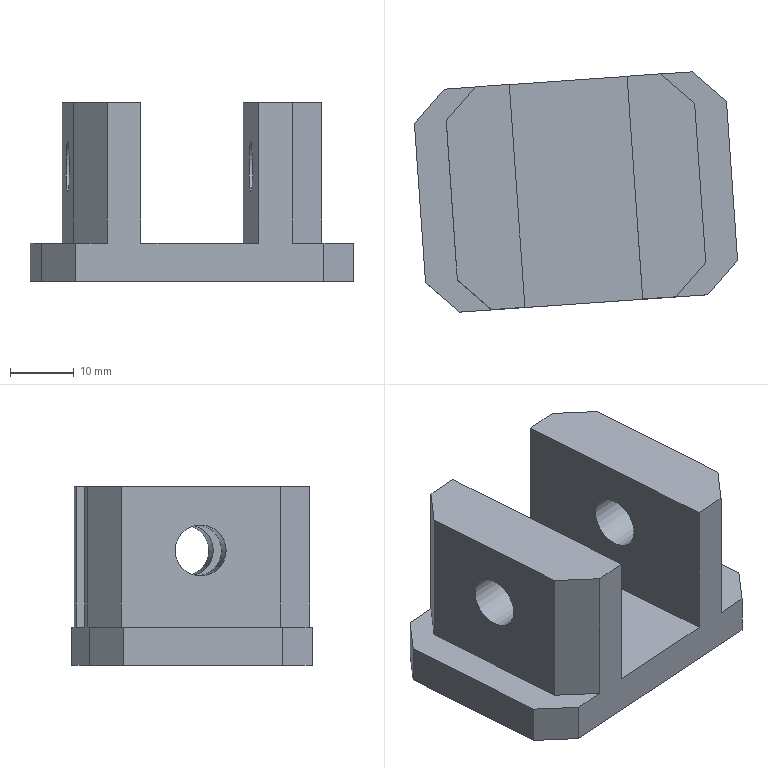Part | STEP file | 车灯-后视镜_id362_x_t | 1 solid | 24 faces | box 50.625 x 37.635 x 28 mm | volume 23645 mm3 | plane 22 | cylinder 2 | commonest cylinder face diameters 8 x2
STEP:
#1=CARTESIAN_POINT('',(14.203,-0.1524,-249.5));
#2=VERTEX_POINT('',#1);
#3=CARTESIAN_POINT('',(-4.252,-1.443,-249.5));
#4=VERTEX_POINT('',#3);
#5=CARTESIAN_POINT('',(22.932,0.458,-249.5));
#6=DIRECTION('',(-0.9976,-0.06976,0.));
#7=VECTOR('',#6,1.);
#8=LINE('',#5,#7);
#9=EDGE_CURVE('',#2,#4,#8,.T.);
#10=ORIENTED_EDGE('',*,*,#9,.T.);
#11=CARTESIAN_POINT('',(-1.81,-36.358,-249.5));
#12=VERTEX_POINT('',#11);
#13=CARTESIAN_POINT('',(-3.417,-13.382,-249.5));
#14=DIRECTION('',(-0.06976,0.9976,0.));
#15=VECTOR('',#14,1.);
#16=LINE('',#13,#15);
#17=EDGE_CURVE('',#12,#4,#16,.T.);
#18=ORIENTED_EDGE('',*,*,#17,.F.);
#19=CARTESIAN_POINT('',(16.645,-35.067,-249.5));
#20=VERTEX_POINT('',#19);
#21=CARTESIAN_POINT('',(25.373,-34.457,-249.5));
#22=DIRECTION('',(0.9976,0.06976,0.));
#23=VECTOR('',#22,1.);
#24=LINE('',#21,#23);
#25=EDGE_CURVE('',#12,#20,#24,.T.);
#26=ORIENTED_EDGE('',*,*,#25,.T.);
#27=CARTESIAN_POINT('',(15.038,-12.092,-249.5));
#28=DIRECTION('',(0.06976,-0.9976,0.));
#29=VECTOR('',#28,1.);
#30=LINE('',#27,#29);
#31=EDGE_CURVE('',#2,#20,#30,.T.);
#32=ORIENTED_EDGE('',*,*,#31,.F.);
#33=EDGE_LOOP('',(#10,#18,#26,#32));
#34=FACE_OUTER_BOUND('',#33,.T.);
#35=CARTESIAN_POINT('',(23.294,-4.723,-249.5));
#36=DIRECTION('',(0.,0.,1.));
#37=DIRECTION('',(0.06976,-0.9976,0.));
#38=AXIS2_PLACEMENT_3D('',#35,#36,#37);
#39=PLANE('',#38);
#40=ADVANCED_FACE('',(#34),#39,.T.);
#41=CARTESIAN_POINT('',(24.428,0.5626,-249.5));
#42=VERTEX_POINT('',#41);
#43=CARTESIAN_POINT('',(19.44,0.2139,-249.5));
#44=VERTEX_POINT('',#43);
#45=CARTESIAN_POINT('',(11.959,-0.3093,-249.5));
#46=DIRECTION('',(-0.9976,-0.06976,0.));
#47=VECTOR('',#46,1.);
#48=LINE('',#45,#47);
#49=EDGE_CURVE('',#42,#44,#48,.T.);
#50=ORIENTED_EDGE('',*,*,#49,.T.);
#51=CARTESIAN_POINT('',(24.777,-4.425,-249.5));
#52=VERTEX_POINT('',#51);
#53=CARTESIAN_POINT('',(19.44,0.2139,-249.5));
#54=DIRECTION('',(-0.7547,0.6561,0.));
#55=VECTOR('',#54,1.);
#56=LINE('',#53,#55);
#57=EDGE_CURVE('',#52,#44,#56,.T.);
#58=ORIENTED_EDGE('',*,*,#57,.F.);
#59=CARTESIAN_POINT('',(26.521,-29.364,-249.5));
#60=VERTEX_POINT('',#59);
#61=CARTESIAN_POINT('',(25.589,-16.037,-249.5));
#62=DIRECTION('',(-0.06976,0.9976,0.));
#63=VECTOR('',#62,1.);
#64=LINE('',#61,#63);
#65=EDGE_CURVE('',#60,#52,#64,.T.);
#66=ORIENTED_EDGE('',*,*,#65,.F.);
#67=CARTESIAN_POINT('',(21.882,-34.701,-249.5));
#68=VERTEX_POINT('',#67);
#69=CARTESIAN_POINT('',(26.521,-29.364,-249.5));
#70=DIRECTION('',(0.6561,0.7547,0.));
#71=VECTOR('',#70,1.);
#72=LINE('',#69,#71);
#73=EDGE_CURVE('',#68,#60,#72,.T.);
#74=ORIENTED_EDGE('',*,*,#73,.F.);
#75=CARTESIAN_POINT('',(26.87,-34.352,-249.5));
#76=VERTEX_POINT('',#75);
#77=CARTESIAN_POINT('',(14.4,-35.224,-249.5));
#78=DIRECTION('',(0.9976,0.06976,0.));
#79=VECTOR('',#78,1.);
#80=LINE('',#77,#79);
#81=EDGE_CURVE('',#68,#76,#80,.T.);
#82=ORIENTED_EDGE('',*,*,#81,.T.);
#83=CARTESIAN_POINT('',(31.509,-29.015,-249.5));
#84=VERTEX_POINT('',#83);
#85=CARTESIAN_POINT('',(31.509,-29.015,-249.5));
#86=DIRECTION('',(-0.6561,-0.7547,0.));
#87=VECTOR('',#86,1.);
#88=LINE('',#85,#87);
#89=EDGE_CURVE('',#84,#76,#88,.T.);
#90=ORIENTED_EDGE('',*,*,#89,.F.);
#91=CARTESIAN_POINT('',(29.765,-4.076,-249.5));
#92=VERTEX_POINT('',#91);
#93=CARTESIAN_POINT('',(29.778,-4.269,-249.5));
#94=DIRECTION('',(-0.06976,0.9976,0.));
#95=VECTOR('',#94,1.);
#96=LINE('',#93,#95);
#97=EDGE_CURVE('',#84,#92,#96,.T.);
#98=ORIENTED_EDGE('',*,*,#97,.T.);
#99=CARTESIAN_POINT('',(24.428,0.5626,-249.5));
#100=DIRECTION('',(0.7547,-0.6561,0.));
#101=VECTOR('',#100,1.);
#102=LINE('',#99,#101);
#103=EDGE_CURVE('',#42,#92,#102,.T.);
#104=ORIENTED_EDGE('',*,*,#103,.F.);
#105=EDGE_LOOP('',(#50,#58,#66,#74,#82,#90,#98,#104));
#106=FACE_OUTER_BOUND('',#105,.T.);
#107=CARTESIAN_POINT('',(12.321,-5.49,-249.5));
#108=DIRECTION('',(0.,0.,1.));
#109=DIRECTION('',(0.06976,-0.9976,0.));
#110=AXIS2_PLACEMENT_3D('',#107,#108,#109);
#111=PLANE('',#110);
#112=ADVANCED_FACE('',(#106),#111,.T.);
#113=CARTESIAN_POINT('',(-19.116,-7.494,-249.5));
#114=VERTEX_POINT('',#113);
#115=CARTESIAN_POINT('',(-17.372,-32.434,-249.5));
#116=VERTEX_POINT('',#115);
#117=CARTESIAN_POINT('',(-19.102,-7.687,-249.5));
#118=DIRECTION('',(0.06976,-0.9976,0.));
#119=VECTOR('',#118,1.);
#120=LINE('',#117,#119);
#121=EDGE_CURVE('',#114,#116,#120,.T.);
#122=ORIENTED_EDGE('',*,*,#121,.T.);
#123=CARTESIAN_POINT('',(-12.035,-37.073,-249.5));
#124=VERTEX_POINT('',#123);
#125=CARTESIAN_POINT('',(-12.035,-37.073,-249.5));
#126=DIRECTION('',(-0.7547,0.6561,0.));
#127=VECTOR('',#126,1.);
#128=LINE('',#125,#127);
#129=EDGE_CURVE('',#124,#116,#128,.T.);
#130=ORIENTED_EDGE('',*,*,#129,.F.);
#131=CARTESIAN_POINT('',(-7.048,-36.724,-249.5));
#132=VERTEX_POINT('',#131);
#133=CARTESIAN_POINT('',(35.349,-33.759,-249.5));
#134=DIRECTION('',(0.9976,0.06976,0.));
#135=VECTOR('',#134,1.);
#136=LINE('',#133,#135);
#137=EDGE_CURVE('',#124,#132,#136,.T.);
#138=ORIENTED_EDGE('',*,*,#137,.T.);
#139=CARTESIAN_POINT('',(-12.384,-32.085,-249.5));
#140=VERTEX_POINT('',#139);
#141=CARTESIAN_POINT('',(-7.048,-36.724,-249.5));
#142=DIRECTION('',(0.7547,-0.6561,0.));
#143=VECTOR('',#142,1.);
#144=LINE('',#141,#143);
#145=EDGE_CURVE('',#140,#132,#144,.T.);
#146=ORIENTED_EDGE('',*,*,#145,.F.);
#147=CARTESIAN_POINT('',(-14.128,-7.146,-249.5));
#148=VERTEX_POINT('',#147);
#149=CARTESIAN_POINT('',(-13.316,-18.757,-249.5));
#150=DIRECTION('',(0.06976,-0.9976,0.));
#151=VECTOR('',#150,1.);
#152=LINE('',#149,#151);
#153=EDGE_CURVE('',#148,#140,#152,.T.);
#154=ORIENTED_EDGE('',*,*,#153,.F.);
#155=CARTESIAN_POINT('',(-9.489,-1.809,-249.5));
#156=VERTEX_POINT('',#155);
#157=CARTESIAN_POINT('',(-14.128,-7.146,-249.5));
#158=DIRECTION('',(-0.6561,-0.7547,0.));
#159=VECTOR('',#158,1.);
#160=LINE('',#157,#159);
#161=EDGE_CURVE('',#156,#148,#160,.T.);
#162=ORIENTED_EDGE('',*,*,#161,.F.);
#163=CARTESIAN_POINT('',(-14.477,-2.158,-249.5));
#164=VERTEX_POINT('',#163);
#165=CARTESIAN_POINT('',(32.907,1.156,-249.5));
#166=DIRECTION('',(-0.9976,-0.06976,0.));
#167=VECTOR('',#166,1.);
#168=LINE('',#165,#167);
#169=EDGE_CURVE('',#156,#164,#168,.T.);
#170=ORIENTED_EDGE('',*,*,#169,.T.);
#171=CARTESIAN_POINT('',(-19.116,-7.494,-249.5));
#172=DIRECTION('',(0.6561,0.7547,0.));
#173=VECTOR('',#172,1.);
#174=LINE('',#171,#173);
#175=EDGE_CURVE('',#114,#164,#174,.T.);
#176=ORIENTED_EDGE('',*,*,#175,.F.);
#177=EDGE_LOOP('',(#122,#130,#138,#146,#154,#162,#170,#176));
#178=FACE_OUTER_BOUND('',#177,.T.);
#179=CARTESIAN_POINT('',(33.27,-4.025,-249.5));
#180=DIRECTION('',(0.,0.,1.));
#181=DIRECTION('',(0.06976,-0.9976,0.));
#182=AXIS2_PLACEMENT_3D('',#179,#180,#181);
#183=PLANE('',#182);
#184=ADVANCED_FACE('',(#178),#183,.T.);
#185=ORIENTED_EDGE('',*,*,#97,.F.);
#186=CARTESIAN_POINT('',(31.509,-29.015,-255.5));
#187=VERTEX_POINT('',#186);
#188=CARTESIAN_POINT('',(31.509,-29.015,-255.5));
#189=DIRECTION('',(0.,0.,1.));
#190=VECTOR('',#189,1.);
#191=LINE('',#188,#190);
#192=EDGE_CURVE('',#187,#84,#191,.T.);
#193=ORIENTED_EDGE('',*,*,#192,.F.);
#194=CARTESIAN_POINT('',(29.765,-4.076,-255.5));
#195=VERTEX_POINT('',#194);
#196=CARTESIAN_POINT('',(30.577,-15.688,-255.5));
#197=DIRECTION('',(0.06976,-0.9976,0.));
#198=VECTOR('',#197,1.);
#199=LINE('',#196,#198);
#200=EDGE_CURVE('',#195,#187,#199,.T.);
#201=ORIENTED_EDGE('',*,*,#200,.F.);
#202=CARTESIAN_POINT('',(29.765,-4.076,-255.5));
#203=DIRECTION('',(0.,0.,-1.));
#204=VECTOR('',#203,1.);
#205=LINE('',#202,#204);
#206=EDGE_CURVE('',#92,#195,#205,.T.);
#207=ORIENTED_EDGE('',*,*,#206,.F.);
#208=EDGE_LOOP('',(#185,#193,#201,#207));
#209=FACE_OUTER_BOUND('',#208,.T.);
#210=CARTESIAN_POINT('',(30.577,-15.688,-255.5));
#211=DIRECTION('',(0.9976,0.06976,0.));
#212=DIRECTION('',(0.,0.,-1.));
#213=AXIS2_PLACEMENT_3D('',#210,#211,#212);
#214=PLANE('',#213);
#215=ADVANCED_FACE('',(#209),#214,.T.);
#216=CARTESIAN_POINT('',(-14.477,-2.158,-255.5));
#217=VERTEX_POINT('',#216);
#218=CARTESIAN_POINT('',(24.428,0.5626,-255.5));
#219=VERTEX_POINT('',#218);
#220=CARTESIAN_POINT('',(-6.995,-1.635,-255.5));
#221=DIRECTION('',(0.9976,0.06976,0.));
#222=VECTOR('',#221,1.);
#223=LINE('',#220,#222);
#224=EDGE_CURVE('',#217,#219,#223,.T.);
#225=ORIENTED_EDGE('',*,*,#224,.F.);
#226=CARTESIAN_POINT('',(-14.477,-2.158,-255.5));
#227=DIRECTION('',(0.,0.,-1.));
#228=VECTOR('',#227,1.);
#229=LINE('',#226,#228);
#230=EDGE_CURVE('',#164,#217,#229,.T.);
#231=ORIENTED_EDGE('',*,*,#230,.F.);
#232=ORIENTED_EDGE('',*,*,#169,.F.);
#233=CARTESIAN_POINT('',(-9.489,-1.809,-227.5));
#234=VERTEX_POINT('',#233);
#235=CARTESIAN_POINT('',(-9.489,-1.809,-255.5));
#236=DIRECTION('',(0.,0.,-1.));
#237=VECTOR('',#236,1.);
#238=LINE('',#235,#237);
#239=EDGE_CURVE('',#234,#156,#238,.T.);
#240=ORIENTED_EDGE('',*,*,#239,.F.);
#241=CARTESIAN_POINT('',(-4.252,-1.443,-227.5));
#242=VERTEX_POINT('',#241);
#243=CARTESIAN_POINT('',(-4.002,-1.425,-227.5));
#244=DIRECTION('',(-0.9976,-0.06976,0.));
#245=VECTOR('',#244,1.);
#246=LINE('',#243,#245);
#247=EDGE_CURVE('',#242,#234,#246,.T.);
#248=ORIENTED_EDGE('',*,*,#247,.F.);
#249=CARTESIAN_POINT('',(-4.252,-1.443,-255.5));
#250=DIRECTION('',(0.,0.,-1.));
#251=VECTOR('',#250,1.);
#252=LINE('',#249,#251);
#253=EDGE_CURVE('',#242,#4,#252,.T.);
#254=ORIENTED_EDGE('',*,*,#253,.T.);
#255=ORIENTED_EDGE('',*,*,#9,.F.);
#256=CARTESIAN_POINT('',(14.203,-0.1524,-227.5));
#257=VERTEX_POINT('',#256);
#258=CARTESIAN_POINT('',(14.203,-0.1524,-243.));
#259=DIRECTION('',(0.,0.,-1.));
#260=VECTOR('',#259,1.);
#261=LINE('',#258,#260);
#262=EDGE_CURVE('',#257,#2,#261,.T.);
#263=ORIENTED_EDGE('',*,*,#262,.F.);
#264=CARTESIAN_POINT('',(19.44,0.2139,-227.5));
#265=VERTEX_POINT('',#264);
#266=CARTESIAN_POINT('',(-10.985,-1.914,-227.5));
#267=DIRECTION('',(-0.9976,-0.06976,0.));
#268=VECTOR('',#267,1.);
#269=LINE('',#266,#268);
#270=EDGE_CURVE('',#265,#257,#269,.T.);
#271=ORIENTED_EDGE('',*,*,#270,.F.);
#272=CARTESIAN_POINT('',(19.44,0.2139,-255.5));
#273=DIRECTION('',(0.,0.,1.));
#274=VECTOR('',#273,1.);
#275=LINE('',#272,#274);
#276=EDGE_CURVE('',#44,#265,#275,.T.);
#277=ORIENTED_EDGE('',*,*,#276,.F.);
#278=ORIENTED_EDGE('',*,*,#49,.F.);
#279=CARTESIAN_POINT('',(24.428,0.5626,-255.5));
#280=DIRECTION('',(0.,0.,1.));
#281=VECTOR('',#280,1.);
#282=LINE('',#279,#281);
#283=EDGE_CURVE('',#219,#42,#282,.T.);
#284=ORIENTED_EDGE('',*,*,#283,.F.);
#285=EDGE_LOOP('',(#225,#231,#232,#240,#248,#254,#255,#263,#271,#277,#278,#284));
#286=FACE_OUTER_BOUND('',#285,.T.);
#287=CARTESIAN_POINT('',(-6.995,-1.635,-255.5));
#288=DIRECTION('',(-0.06976,0.9976,0.));
#289=DIRECTION('',(0.,0.,1.));
#290=AXIS2_PLACEMENT_3D('',#287,#288,#289);
#291=PLANE('',#290);
#292=ADVANCED_FACE('',(#286),#291,.T.);
#293=CARTESIAN_POINT('',(-17.372,-32.434,-255.5));
#294=VERTEX_POINT('',#293);
#295=CARTESIAN_POINT('',(-19.116,-7.494,-255.5));
#296=VERTEX_POINT('',#295);
#297=CARTESIAN_POINT('',(-18.304,-19.106,-255.5));
#298=DIRECTION('',(-0.06976,0.9976,0.));
#299=VECTOR('',#298,1.);
#300=LINE('',#297,#299);
#301=EDGE_CURVE('',#294,#296,#300,.T.);
#302=ORIENTED_EDGE('',*,*,#301,.F.);
#303=CARTESIAN_POINT('',(-17.372,-32.434,-255.5));
#304=DIRECTION('',(0.,0.,-1.));
#305=VECTOR('',#304,1.);
#306=LINE('',#303,#305);
#307=EDGE_CURVE('',#116,#294,#306,.T.);
#308=ORIENTED_EDGE('',*,*,#307,.F.);
#309=ORIENTED_EDGE('',*,*,#121,.F.);
#310=CARTESIAN_POINT('',(-19.116,-7.494,-255.5));
#311=DIRECTION('',(0.,0.,1.));
#312=VECTOR('',#311,1.);
#313=LINE('',#310,#312);
#314=EDGE_CURVE('',#296,#114,#313,.T.);
#315=ORIENTED_EDGE('',*,*,#314,.F.);
#316=EDGE_LOOP('',(#302,#308,#309,#315));
#317=FACE_OUTER_BOUND('',#316,.T.);
#318=CARTESIAN_POINT('',(-18.304,-19.106,-255.5));
#319=DIRECTION('',(-0.9976,-0.06976,0.));
#320=DIRECTION('',(0.,0.,1.));
#321=AXIS2_PLACEMENT_3D('',#318,#319,#320);
#322=PLANE('',#321);
#323=ADVANCED_FACE('',(#317),#322,.T.);
#324=ORIENTED_EDGE('',*,*,#81,.F.);
#325=CARTESIAN_POINT('',(21.882,-34.701,-227.5));
#326=VERTEX_POINT('',#325);
#327=CARTESIAN_POINT('',(21.882,-34.701,-255.5));
#328=DIRECTION('',(0.,0.,-1.));
#329=VECTOR('',#328,1.);
#330=LINE('',#327,#329);
#331=EDGE_CURVE('',#326,#68,#330,.T.);
#332=ORIENTED_EDGE('',*,*,#331,.F.);
#333=CARTESIAN_POINT('',(16.645,-35.067,-227.5));
#334=VERTEX_POINT('',#333);
#335=CARTESIAN_POINT('',(-8.544,-36.828,-227.5));
#336=DIRECTION('',(0.9976,0.06976,0.));
#337=VECTOR('',#336,1.);
#338=LINE('',#335,#337);
#339=EDGE_CURVE('',#334,#326,#338,.T.);
#340=ORIENTED_EDGE('',*,*,#339,.F.);
#341=CARTESIAN_POINT('',(16.645,-35.067,-243.));
#342=DIRECTION('',(0.,0.,1.));
#343=VECTOR('',#342,1.);
#344=LINE('',#341,#343);
#345=EDGE_CURVE('',#20,#334,#344,.T.);
#346=ORIENTED_EDGE('',*,*,#345,.F.);
#347=ORIENTED_EDGE('',*,*,#25,.F.);
#348=CARTESIAN_POINT('',(-1.81,-36.358,-227.5));
#349=VERTEX_POINT('',#348);
#350=CARTESIAN_POINT('',(-1.81,-36.358,-255.5));
#351=DIRECTION('',(0.,0.,1.));
#352=VECTOR('',#351,1.);
#353=LINE('',#350,#352);
#354=EDGE_CURVE('',#12,#349,#353,.T.);
#355=ORIENTED_EDGE('',*,*,#354,.T.);
#356=CARTESIAN_POINT('',(-7.048,-36.724,-227.5));
#357=VERTEX_POINT('',#356);
#358=CARTESIAN_POINT('',(-1.561,-36.34,-227.5));
#359=DIRECTION('',(0.9976,0.06976,0.));
#360=VECTOR('',#359,1.);
#361=LINE('',#358,#360);
#362=EDGE_CURVE('',#357,#349,#361,.T.);
#363=ORIENTED_EDGE('',*,*,#362,.F.);
#364=CARTESIAN_POINT('',(-7.048,-36.724,-255.5));
#365=DIRECTION('',(0.,0.,1.));
#366=VECTOR('',#365,1.);
#367=LINE('',#364,#366);
#368=EDGE_CURVE('',#132,#357,#367,.T.);
#369=ORIENTED_EDGE('',*,*,#368,.F.);
#370=ORIENTED_EDGE('',*,*,#137,.F.);
#371=CARTESIAN_POINT('',(-12.035,-37.073,-255.5));
#372=VERTEX_POINT('',#371);
#373=CARTESIAN_POINT('',(-12.035,-37.073,-255.5));
#374=DIRECTION('',(0.,0.,1.));
#375=VECTOR('',#374,1.);
#376=LINE('',#373,#375);
#377=EDGE_CURVE('',#372,#124,#376,.T.);
#378=ORIENTED_EDGE('',*,*,#377,.F.);
#379=CARTESIAN_POINT('',(26.87,-34.352,-255.5));
#380=VERTEX_POINT('',#379);
#381=CARTESIAN_POINT('',(-4.554,-36.549,-255.5));
#382=DIRECTION('',(-0.9976,-0.06976,0.));
#383=VECTOR('',#382,1.);
#384=LINE('',#381,#383);
#385=EDGE_CURVE('',#380,#372,#384,.T.);
#386=ORIENTED_EDGE('',*,*,#385,.F.);
#387=CARTESIAN_POINT('',(26.87,-34.352,-255.5));
#388=DIRECTION('',(0.,0.,-1.));
#389=VECTOR('',#388,1.);
#390=LINE('',#387,#389);
#391=EDGE_CURVE('',#76,#380,#390,.T.);
#392=ORIENTED_EDGE('',*,*,#391,.F.);
#393=EDGE_LOOP('',(#324,#332,#340,#346,#347,#355,#363,#369,#370,#378,#386,#392));
#394=FACE_OUTER_BOUND('',#393,.T.);
#395=CARTESIAN_POINT('',(-4.554,-36.549,-255.5));
#396=DIRECTION('',(0.06976,-0.9976,0.));
#397=DIRECTION('',(0.,0.,-1.));
#398=AXIS2_PLACEMENT_3D('',#395,#396,#397);
#399=PLANE('',#398);
#400=ADVANCED_FACE('',(#394),#399,.T.);
#401=ORIENTED_EDGE('',*,*,#200,.T.);
#402=CARTESIAN_POINT('',(31.509,-29.015,-255.5));
#403=DIRECTION('',(0.6561,0.7547,0.));
#404=VECTOR('',#403,1.);
#405=LINE('',#402,#404);
#406=EDGE_CURVE('',#380,#187,#405,.T.);
#407=ORIENTED_EDGE('',*,*,#406,.F.);
#408=ORIENTED_EDGE('',*,*,#385,.T.);
#409=CARTESIAN_POINT('',(-12.035,-37.073,-255.5));
#410=DIRECTION('',(0.7547,-0.6561,0.));
#411=VECTOR('',#410,1.);
#412=LINE('',#409,#411);
#413=EDGE_CURVE('',#294,#372,#412,.T.);
#414=ORIENTED_EDGE('',*,*,#413,.F.);
#415=ORIENTED_EDGE('',*,*,#301,.T.);
#416=CARTESIAN_POINT('',(-19.116,-7.494,-255.5));
#417=DIRECTION('',(-0.6561,-0.7547,0.));
#418=VECTOR('',#417,1.);
#419=LINE('',#416,#418);
#420=EDGE_CURVE('',#217,#296,#419,.T.);
#421=ORIENTED_EDGE('',*,*,#420,.F.);
#422=ORIENTED_EDGE('',*,*,#224,.T.);
#423=CARTESIAN_POINT('',(24.428,0.5626,-255.5));
#424=DIRECTION('',(-0.7547,0.6561,0.));
#425=VECTOR('',#424,1.);
#426=LINE('',#423,#425);
#427=EDGE_CURVE('',#195,#219,#426,.T.);
#428=ORIENTED_EDGE('',*,*,#427,.F.);
#429=EDGE_LOOP('',(#401,#407,#408,#414,#415,#421,#422,#428));
#430=FACE_OUTER_BOUND('',#429,.T.);
#431=CARTESIAN_POINT('',(-5.834,-18.234,-255.5));
#432=DIRECTION('',(0.,0.,-1.));
#433=DIRECTION('',(-0.06976,0.9976,0.));
#434=AXIS2_PLACEMENT_3D('',#431,#432,#433);
#435=PLANE('',#434);
#436=ADVANCED_FACE('',(#430),#435,.T.);
#437=CARTESIAN_POINT('',(-12.977,-23.605,-237.501));
#438=VERTEX_POINT('',#437);
#439=CARTESIAN_POINT('',(-13.256,-19.615,-237.501));
#440=DIRECTION('',(0.9976,0.06976,0.));
#441=DIRECTION('',(0.06976,-0.9976,0.));
#442=AXIS2_PLACEMENT_3D('',#439,#440,#441);
#443=CIRCLE('',#442,4.);
#444=EDGE_CURVE('',#438,#438,#443,.T.);
#445=ORIENTED_EDGE('',*,*,#444,.T.);
#446=EDGE_LOOP('',(#445));
#447=FACE_BOUND('',#446,.T.);
#448=ORIENTED_EDGE('',*,*,#153,.T.);
#449=CARTESIAN_POINT('',(-12.384,-32.085,-227.5));
#450=VERTEX_POINT('',#449);
#451=CARTESIAN_POINT('',(-12.384,-32.085,-255.5));
#452=DIRECTION('',(0.,0.,-1.));
#453=VECTOR('',#452,1.);
#454=LINE('',#451,#453);
#455=EDGE_CURVE('',#450,#140,#454,.T.);
#456=ORIENTED_EDGE('',*,*,#455,.F.);
#457=CARTESIAN_POINT('',(-14.128,-7.146,-227.5));
#458=VERTEX_POINT('',#457);
#459=CARTESIAN_POINT('',(-13.316,-18.757,-227.5));
#460=DIRECTION('',(0.06976,-0.9976,0.));
#461=VECTOR('',#460,1.);
#462=LINE('',#459,#461);
#463=EDGE_CURVE('',#458,#450,#462,.T.);
#464=ORIENTED_EDGE('',*,*,#463,.F.);
#465=CARTESIAN_POINT('',(-14.128,-7.146,-255.5));
#466=DIRECTION('',(0.,0.,1.));
#467=VECTOR('',#466,1.);
#468=LINE('',#465,#467);
#469=EDGE_CURVE('',#148,#458,#468,.T.);
#470=ORIENTED_EDGE('',*,*,#469,.F.);
#471=EDGE_LOOP('',(#448,#456,#464,#470));
#472=FACE_BOUND('',#471,.T.);
#473=CARTESIAN_POINT('',(-13.316,-18.757,-255.5));
#474=DIRECTION('',(-0.9976,-0.06976,0.));
#475=DIRECTION('',(0.,0.,1.));
#476=AXIS2_PLACEMENT_3D('',#473,#474,#475);
#477=PLANE('',#476);
#478=ADVANCED_FACE('',(#447,#472),#477,.T.);
#479=CARTESIAN_POINT('',(-2.752,-22.89,-237.501));
#480=VERTEX_POINT('',#479);
#481=CARTESIAN_POINT('',(-3.031,-18.9,-237.501));
#482=DIRECTION('',(0.9976,0.06976,0.));
#483=DIRECTION('',(0.06976,-0.9976,0.));
#484=AXIS2_PLACEMENT_3D('',#481,#482,#483);
#485=CIRCLE('',#484,4.);
#486=EDGE_CURVE('',#480,#480,#485,.T.);
#487=ORIENTED_EDGE('',*,*,#486,.F.);
#488=EDGE_LOOP('',(#487));
#489=FACE_BOUND('',#488,.T.);
#490=CARTESIAN_POINT('',(-3.091,-18.042,-227.5));
#491=DIRECTION('',(-0.06976,0.9976,0.));
#492=VECTOR('',#491,1.);
#493=LINE('',#490,#492);
#494=EDGE_CURVE('',#349,#242,#493,.T.);
#495=ORIENTED_EDGE('',*,*,#494,.F.);
#496=ORIENTED_EDGE('',*,*,#354,.F.);
#497=ORIENTED_EDGE('',*,*,#17,.T.);
#498=ORIENTED_EDGE('',*,*,#253,.F.);
#499=EDGE_LOOP('',(#495,#496,#497,#498));
#500=FACE_BOUND('',#499,.T.);
#501=CARTESIAN_POINT('',(-3.417,-13.382,-243.));
#502=DIRECTION('',(-0.9976,-0.06976,0.));
#503=DIRECTION('',(0.,0.,1.));
#504=AXIS2_PLACEMENT_3D('',#501,#502,#503);
#505=PLANE('',#504);
#506=ADVANCED_FACE('',(#489,#500),#505,.F.);
#507=ORIENTED_EDGE('',*,*,#463,.T.);
#508=CARTESIAN_POINT('',(-7.048,-36.724,-227.5));
#509=DIRECTION('',(-0.7547,0.6561,0.));
#510=VECTOR('',#509,1.);
#511=LINE('',#508,#510);
#512=EDGE_CURVE('',#357,#450,#511,.T.);
#513=ORIENTED_EDGE('',*,*,#512,.F.);
#514=ORIENTED_EDGE('',*,*,#362,.T.);
#515=ORIENTED_EDGE('',*,*,#494,.T.);
#516=ORIENTED_EDGE('',*,*,#247,.T.);
#517=CARTESIAN_POINT('',(-14.128,-7.146,-227.5));
#518=DIRECTION('',(0.6561,0.7547,0.));
#519=VECTOR('',#518,1.);
#520=LINE('',#517,#519);
#521=EDGE_CURVE('',#458,#234,#520,.T.);
#522=ORIENTED_EDGE('',*,*,#521,.F.);
#523=EDGE_LOOP('',(#507,#513,#514,#515,#516,#522));
#524=FACE_OUTER_BOUND('',#523,.T.);
#525=CARTESIAN_POINT('',(-2.842,-18.025,-227.5));
#526=DIRECTION('',(0.,0.,1.));
#527=DIRECTION('',(0.06976,-0.9976,0.));
#528=AXIS2_PLACEMENT_3D('',#525,#526,#527);
#529=PLANE('',#528);
#530=ADVANCED_FACE('',(#524),#529,.T.);
#531=CARTESIAN_POINT('',(26.521,-29.364,-227.5));
#532=VERTEX_POINT('',#531);
#533=CARTESIAN_POINT('',(24.777,-4.425,-227.5));
#534=VERTEX_POINT('',#533);
#535=CARTESIAN_POINT('',(25.589,-16.037,-227.5));
#536=DIRECTION('',(-0.06976,0.9976,0.));
#537=VECTOR('',#536,1.);
#538=LINE('',#535,#537);
#539=EDGE_CURVE('',#532,#534,#538,.T.);
#540=ORIENTED_EDGE('',*,*,#539,.T.);
#541=CARTESIAN_POINT('',(19.44,0.2139,-227.5));
#542=DIRECTION('',(0.7547,-0.6561,0.));
#543=VECTOR('',#542,1.);
#544=LINE('',#541,#543);
#545=EDGE_CURVE('',#265,#534,#544,.T.);
#546=ORIENTED_EDGE('',*,*,#545,.F.);
#547=ORIENTED_EDGE('',*,*,#270,.T.);
#548=CARTESIAN_POINT('',(15.038,-12.092,-227.5));
#549=DIRECTION('',(-0.06976,0.9976,0.));
#550=VECTOR('',#549,1.);
#551=LINE('',#548,#550);
#552=EDGE_CURVE('',#334,#257,#551,.T.);
#553=ORIENTED_EDGE('',*,*,#552,.F.);
#554=ORIENTED_EDGE('',*,*,#339,.T.);
#555=CARTESIAN_POINT('',(26.521,-29.364,-227.5));
#556=DIRECTION('',(-0.6561,-0.7547,0.));
#557=VECTOR('',#556,1.);
#558=LINE('',#555,#557);
#559=EDGE_CURVE('',#532,#326,#558,.T.);
#560=ORIENTED_EDGE('',*,*,#559,.F.);
#561=EDGE_LOOP('',(#540,#546,#547,#553,#554,#560));
#562=FACE_OUTER_BOUND('',#561,.T.);
#563=CARTESIAN_POINT('',(-9.825,-18.513,-227.5));
#564=DIRECTION('',(0.,0.,1.));
#565=DIRECTION('',(0.06976,-0.9976,0.));
#566=AXIS2_PLACEMENT_3D('',#563,#564,#565);
#567=PLANE('',#566);
#568=ADVANCED_FACE('',(#562),#567,.T.);
#569=CARTESIAN_POINT('',(25.37,-12.904,-237.501));
#570=VERTEX_POINT('',#569);
#571=CARTESIAN_POINT('',(25.649,-16.895,-237.501));
#572=DIRECTION('',(-0.9976,-0.06976,0.));
#573=DIRECTION('',(-0.06976,0.9976,0.));
#574=AXIS2_PLACEMENT_3D('',#571,#572,#573);
#575=CIRCLE('',#574,4.);
#576=EDGE_CURVE('',#570,#570,#575,.T.);
#577=ORIENTED_EDGE('',*,*,#576,.T.);
#578=EDGE_LOOP('',(#577));
#579=FACE_BOUND('',#578,.T.);
#580=ORIENTED_EDGE('',*,*,#65,.T.);
#581=CARTESIAN_POINT('',(24.777,-4.425,-255.5));
#582=DIRECTION('',(0.,0.,-1.));
#583=VECTOR('',#582,1.);
#584=LINE('',#581,#583);
#585=EDGE_CURVE('',#534,#52,#584,.T.);
#586=ORIENTED_EDGE('',*,*,#585,.F.);
#587=ORIENTED_EDGE('',*,*,#539,.F.);
#588=CARTESIAN_POINT('',(26.521,-29.364,-255.5));
#589=DIRECTION('',(0.,0.,1.));
#590=VECTOR('',#589,1.);
#591=LINE('',#588,#590);
#592=EDGE_CURVE('',#60,#532,#591,.T.);
#593=ORIENTED_EDGE('',*,*,#592,.F.);
#594=EDGE_LOOP('',(#580,#586,#587,#593));
#595=FACE_BOUND('',#594,.T.);
#596=CARTESIAN_POINT('',(25.589,-16.037,-255.5));
#597=DIRECTION('',(0.9976,0.06976,0.));
#598=DIRECTION('',(0.,0.,-1.));
#599=AXIS2_PLACEMENT_3D('',#596,#597,#598);
#600=PLANE('',#599);
#601=ADVANCED_FACE('',(#579,#595),#600,.T.);
#602=CARTESIAN_POINT('',(15.145,-13.619,-237.501));
#603=VERTEX_POINT('',#602);
#604=CARTESIAN_POINT('',(15.424,-17.61,-237.501));
#605=DIRECTION('',(-0.9976,-0.06976,0.));
#606=DIRECTION('',(-0.06976,0.9976,0.));
#607=AXIS2_PLACEMENT_3D('',#604,#605,#606);
#608=CIRCLE('',#607,4.);
#609=EDGE_CURVE('',#603,#603,#608,.T.);
#610=ORIENTED_EDGE('',*,*,#609,.F.);
#611=EDGE_LOOP('',(#610));
#612=FACE_BOUND('',#611,.T.);
#613=ORIENTED_EDGE('',*,*,#262,.T.);
#614=ORIENTED_EDGE('',*,*,#31,.T.);
#615=ORIENTED_EDGE('',*,*,#345,.T.);
#616=ORIENTED_EDGE('',*,*,#552,.T.);
#617=EDGE_LOOP('',(#613,#614,#615,#616));
#618=FACE_BOUND('',#617,.T.);
#619=CARTESIAN_POINT('',(15.038,-12.092,-243.));
#620=DIRECTION('',(0.9976,0.06976,0.));
#621=DIRECTION('',(0.,0.,-1.));
#622=AXIS2_PLACEMENT_3D('',#619,#620,#621);
#623=PLANE('',#622);
#624=ADVANCED_FACE('',(#612,#618),#623,.F.);
#625=ORIENTED_EDGE('',*,*,#576,.F.);
#626=EDGE_LOOP('',(#625));
#627=FACE_BOUND('',#626,.T.);
#628=ORIENTED_EDGE('',*,*,#609,.T.);
#629=EDGE_LOOP('',(#628));
#630=FACE_BOUND('',#629,.T.);
#631=CARTESIAN_POINT('',(46.999,-15.402,-237.501));
#632=DIRECTION('',(-0.9976,-0.06976,0.));
#633=DIRECTION('',(0.,0.,1.));
#634=AXIS2_PLACEMENT_3D('',#631,#632,#633);
#635=CYLINDRICAL_SURFACE('',#634,4.);
#636=ADVANCED_FACE('',(#627,#630),#635,.F.);
#637=ORIENTED_EDGE('',*,*,#444,.F.);
#638=EDGE_LOOP('',(#637));
#639=FACE_BOUND('',#638,.T.);
#640=ORIENTED_EDGE('',*,*,#486,.T.);
#641=EDGE_LOOP('',(#640));
#642=FACE_BOUND('',#641,.T.);
#643=CARTESIAN_POINT('',(53.982,-14.913,-237.501));
#644=DIRECTION('',(-0.9976,-0.06976,0.));
#645=DIRECTION('',(0.,0.,1.));
#646=AXIS2_PLACEMENT_3D('',#643,#644,#645);
#647=CYLINDRICAL_SURFACE('',#646,4.);
#648=ADVANCED_FACE('',(#639,#642),#647,.F.);
#649=ORIENTED_EDGE('',*,*,#161,.T.);
#650=ORIENTED_EDGE('',*,*,#469,.T.);
#651=ORIENTED_EDGE('',*,*,#521,.T.);
#652=ORIENTED_EDGE('',*,*,#239,.T.);
#653=EDGE_LOOP('',(#649,#650,#651,#652));
#654=FACE_OUTER_BOUND('',#653,.T.);
#655=CARTESIAN_POINT('',(-14.128,-7.146,-255.5));
#656=DIRECTION('',(0.7547,-0.6561,0.));
#657=DIRECTION('',(-0.6561,-0.7547,0.));
#658=AXIS2_PLACEMENT_3D('',#655,#656,#657);
#659=PLANE('',#658);
#660=ADVANCED_FACE('',(#654),#659,.F.);
#661=ORIENTED_EDGE('',*,*,#145,.T.);
#662=ORIENTED_EDGE('',*,*,#368,.T.);
#663=ORIENTED_EDGE('',*,*,#512,.T.);
#664=ORIENTED_EDGE('',*,*,#455,.T.);
#665=EDGE_LOOP('',(#661,#662,#663,#664));
#666=FACE_OUTER_BOUND('',#665,.T.);
#667=CARTESIAN_POINT('',(-7.048,-36.724,-255.5));
#668=DIRECTION('',(0.6561,0.7547,0.));
#669=DIRECTION('',(0.7547,-0.6561,0.));
#670=AXIS2_PLACEMENT_3D('',#667,#668,#669);
#671=PLANE('',#670);
#672=ADVANCED_FACE('',(#666),#671,.F.);
#673=ORIENTED_EDGE('',*,*,#73,.T.);
#674=ORIENTED_EDGE('',*,*,#592,.T.);
#675=ORIENTED_EDGE('',*,*,#559,.T.);
#676=ORIENTED_EDGE('',*,*,#331,.T.);
#677=EDGE_LOOP('',(#673,#674,#675,#676));
#678=FACE_OUTER_BOUND('',#677,.T.);
#679=CARTESIAN_POINT('',(26.521,-29.364,-255.5));
#680=DIRECTION('',(-0.7547,0.6561,0.));
#681=DIRECTION('',(0.6561,0.7547,0.));
#682=AXIS2_PLACEMENT_3D('',#679,#680,#681);
#683=PLANE('',#682);
#684=ADVANCED_FACE('',(#678),#683,.F.);
#685=ORIENTED_EDGE('',*,*,#57,.T.);
#686=ORIENTED_EDGE('',*,*,#276,.T.);
#687=ORIENTED_EDGE('',*,*,#545,.T.);
#688=ORIENTED_EDGE('',*,*,#585,.T.);
#689=EDGE_LOOP('',(#685,#686,#687,#688));
#690=FACE_OUTER_BOUND('',#689,.T.);
#691=CARTESIAN_POINT('',(19.44,0.2139,-255.5));
#692=DIRECTION('',(-0.6561,-0.7547,0.));
#693=DIRECTION('',(-0.7547,0.6561,0.));
#694=AXIS2_PLACEMENT_3D('',#691,#692,#693);
#695=PLANE('',#694);
#696=ADVANCED_FACE('',(#690),#695,.F.);
#697=ORIENTED_EDGE('',*,*,#427,.T.);
#698=ORIENTED_EDGE('',*,*,#283,.T.);
#699=ORIENTED_EDGE('',*,*,#103,.T.);
#700=ORIENTED_EDGE('',*,*,#206,.T.);
#701=EDGE_LOOP('',(#697,#698,#699,#700));
#702=FACE_OUTER_BOUND('',#701,.T.);
#703=CARTESIAN_POINT('',(24.428,0.5626,-255.5));
#704=DIRECTION('',(-0.6561,-0.7547,0.));
#705=DIRECTION('',(-0.7547,0.6561,0.));
#706=AXIS2_PLACEMENT_3D('',#703,#704,#705);
#707=PLANE('',#706);
#708=ADVANCED_FACE('',(#702),#707,.F.);
#709=ORIENTED_EDGE('',*,*,#406,.T.);
#710=ORIENTED_EDGE('',*,*,#192,.T.);
#711=ORIENTED_EDGE('',*,*,#89,.T.);
#712=ORIENTED_EDGE('',*,*,#391,.T.);
#713=EDGE_LOOP('',(#709,#710,#711,#712));
#714=FACE_OUTER_BOUND('',#713,.T.);
#715=CARTESIAN_POINT('',(31.509,-29.015,-255.5));
#716=DIRECTION('',(-0.7547,0.6561,0.));
#717=DIRECTION('',(0.6561,0.7547,0.));
#718=AXIS2_PLACEMENT_3D('',#715,#716,#717);
#719=PLANE('',#718);
#720=ADVANCED_FACE('',(#714),#719,.F.);
#721=ORIENTED_EDGE('',*,*,#420,.T.);
#722=ORIENTED_EDGE('',*,*,#314,.T.);
#723=ORIENTED_EDGE('',*,*,#175,.T.);
#724=ORIENTED_EDGE('',*,*,#230,.T.);
#725=EDGE_LOOP('',(#721,#722,#723,#724));
#726=FACE_OUTER_BOUND('',#725,.T.);
#727=CARTESIAN_POINT('',(-19.116,-7.494,-255.5));
#728=DIRECTION('',(0.7547,-0.6561,0.));
#729=DIRECTION('',(-0.6561,-0.7547,0.));
#730=AXIS2_PLACEMENT_3D('',#727,#728,#729);
#731=PLANE('',#730);
#732=ADVANCED_FACE('',(#726),#731,.F.);
#733=ORIENTED_EDGE('',*,*,#413,.T.);
#734=ORIENTED_EDGE('',*,*,#377,.T.);
#735=ORIENTED_EDGE('',*,*,#129,.T.);
#736=ORIENTED_EDGE('',*,*,#307,.T.);
#737=EDGE_LOOP('',(#733,#734,#735,#736));
#738=FACE_OUTER_BOUND('',#737,.T.);
#739=CARTESIAN_POINT('',(-12.035,-37.073,-255.5));
#740=DIRECTION('',(0.6561,0.7547,0.));
#741=DIRECTION('',(0.7547,-0.6561,0.));
#742=AXIS2_PLACEMENT_3D('',#739,#740,#741);
#743=PLANE('',#742);
#744=ADVANCED_FACE('',(#738),#743,.F.);
#745=CLOSED_SHELL('',(#40,#112,#184,#215,#292,#323,#400,#436,#478,#506,#530,#568,#601,#624,#636,#648,#660,#672,#684,#696,#708,#720,#732,#744));
#746=MANIFOLD_SOLID_BREP('',#745);
#747=(LENGTH_UNIT()NAMED_UNIT(*)SI_UNIT(.MILLI.,.METRE.));
#748=UNCERTAINTY_MEASURE_WITH_UNIT(LENGTH_MEASURE(0.00002),#747,'','');
#749=(NAMED_UNIT(*)PLANE_ANGLE_UNIT()SI_UNIT($,.RADIAN.));
#750=PLANE_ANGLE_MEASURE_WITH_UNIT(PLANE_ANGLE_MEASURE(0.01745),#749);
#751=DIMENSIONAL_EXPONENTS(0.,0.,0.,0.,0.,0.,0.);
#752=(CONVERSION_BASED_UNIT('DEGREE',#750)NAMED_UNIT(#751)PLANE_ANGLE_UNIT());
#753=(NAMED_UNIT(*)SI_UNIT($,.STERADIAN.)SOLID_ANGLE_UNIT());
#754=(GEOMETRIC_REPRESENTATION_CONTEXT(3)GLOBAL_UNCERTAINTY_ASSIGNED_CONTEXT((#748))GLOBAL_UNIT_ASSIGNED_CONTEXT((#747,#752,#753))REPRESENTATION_CONTEXT('',''));
#755=ADVANCED_BREP_SHAPE_REPRESENTATION('',(#746),#754);